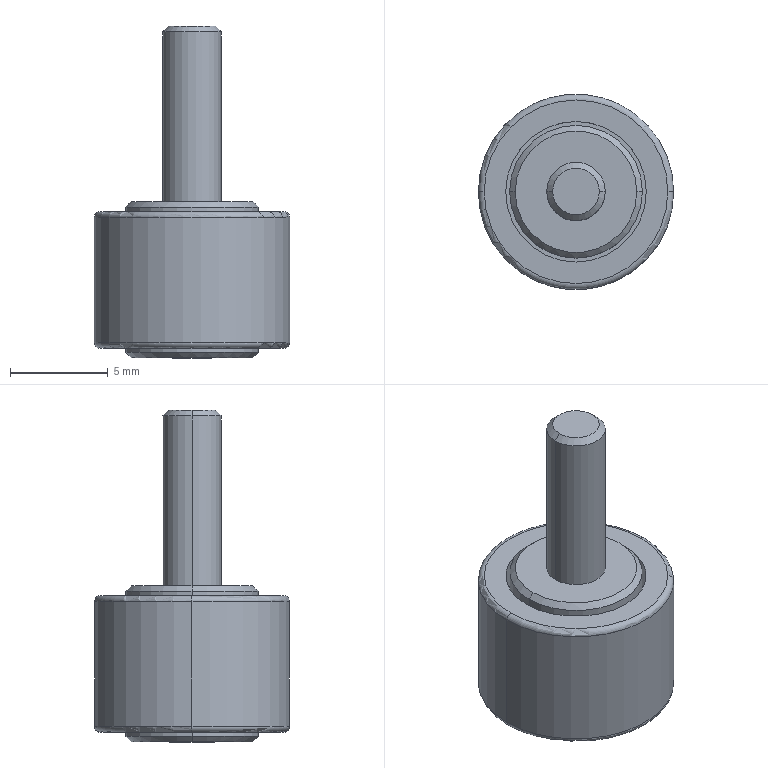Part | NX | features BREP 1 | 1 solid | 36 faces | box 10 x 10 x 17 mm | volume 619.39 mm3 | plane 14 | cylinder 12 | cone 6 | torus 4 | commonest cylinder face diameters 6.8 x4 7.2 x4 3 x2 10 x2
STEP:
#1=CARTESIAN_POINT('',(3.117,0.,-17.));
#2=VERTEX_POINT('',#1);
#3=CARTESIAN_POINT('',(-3.117,0.,-17.));
#4=VERTEX_POINT('',#3);
#5=CARTESIAN_POINT('',(0.,0.,-17.));
#6=DIRECTION('',(0.,0.,1.));
#7=DIRECTION('',(1.,0.,0.));
#8=AXIS2_PLACEMENT_3D('',#5,#6,#7);
#9=CIRCLE('',#8,3.117);
#10=EDGE_CURVE('',#2,#4,#9,.T.);
#11=ORIENTED_EDGE('',*,*,#10,.T.);
#12=CARTESIAN_POINT('',(-3.4,0.,-16.717));
#13=VERTEX_POINT('',#12);
#14=CARTESIAN_POINT('',(-3.117,0.,-17.));
#15=DIRECTION('',(-0.7071,0.,0.7071));
#16=VECTOR('',#15,1000.);
#17=LINE('',#14,#16);
#18=EDGE_CURVE('',#4,#13,#17,.T.);
#19=ORIENTED_EDGE('',*,*,#18,.T.);
#20=CARTESIAN_POINT('',(3.4,0.,-16.717));
#21=VERTEX_POINT('',#20);
#22=CARTESIAN_POINT('',(0.,0.,-16.717));
#23=DIRECTION('',(0.,0.,1.));
#24=DIRECTION('',(1.,0.,0.));
#25=AXIS2_PLACEMENT_3D('',#22,#23,#24);
#26=CIRCLE('',#25,3.4);
#27=EDGE_CURVE('',#21,#13,#26,.T.);
#28=ORIENTED_EDGE('',*,*,#27,.F.);
#29=CARTESIAN_POINT('',(3.117,0.,-17.));
#30=DIRECTION('',(0.7071,0.,0.7071));
#31=VECTOR('',#30,1000.);
#32=LINE('',#29,#31);
#33=EDGE_CURVE('',#2,#21,#32,.T.);
#34=ORIENTED_EDGE('',*,*,#33,.F.);
#35=EDGE_LOOP('',(#11,#19,#28,#34));
#36=FACE_BOUND('',#35,.T.);
#37=CARTESIAN_POINT('',(0.,0.,-17.));
#38=DIRECTION('',(0.,0.,1.));
#39=DIRECTION('',(-1.,0.,0.));
#40=AXIS2_PLACEMENT_3D('',#37,#38,#39);
#41=CONICAL_SURFACE('',#40,3.117,0.7854);
#42=ADVANCED_FACE('',(#36),#41,.T.);
#43=ORIENTED_EDGE('',*,*,#27,.T.);
#44=CARTESIAN_POINT('',(-3.4,0.,-15.));
#45=VERTEX_POINT('',#44);
#46=CARTESIAN_POINT('',(-3.4,0.,-17.));
#47=DIRECTION('',(0.,0.,1.));
#48=VECTOR('',#47,1000.);
#49=LINE('',#46,#48);
#50=EDGE_CURVE('',#13,#45,#49,.T.);
#51=ORIENTED_EDGE('',*,*,#50,.T.);
#52=CARTESIAN_POINT('',(3.4,0.,-15.));
#53=VERTEX_POINT('',#52);
#54=CARTESIAN_POINT('',(0.,0.,-15.));
#55=DIRECTION('',(0.,0.,1.));
#56=DIRECTION('',(1.,0.,0.));
#57=AXIS2_PLACEMENT_3D('',#54,#55,#56);
#58=CIRCLE('',#57,3.4);
#59=EDGE_CURVE('',#53,#45,#58,.T.);
#60=ORIENTED_EDGE('',*,*,#59,.F.);
#61=CARTESIAN_POINT('',(3.4,0.,-17.));
#62=DIRECTION('',(0.,0.,1.));
#63=VECTOR('',#62,1000.);
#64=LINE('',#61,#63);
#65=EDGE_CURVE('',#21,#53,#64,.T.);
#66=ORIENTED_EDGE('',*,*,#65,.F.);
#67=EDGE_LOOP('',(#43,#51,#60,#66));
#68=FACE_BOUND('',#67,.T.);
#69=CARTESIAN_POINT('',(0.,0.,-17.));
#70=DIRECTION('',(0.,0.,1.));
#71=DIRECTION('',(-1.,0.,0.));
#72=AXIS2_PLACEMENT_3D('',#69,#70,#71);
#73=CYLINDRICAL_SURFACE('',#72,3.4);
#74=ADVANCED_FACE('',(#68),#73,.T.);
#75=CARTESIAN_POINT('',(-3.6,0.,-16.5));
#76=VERTEX_POINT('',#75);
#77=CARTESIAN_POINT('',(3.6,0.,-16.5));
#78=VERTEX_POINT('',#77);
#79=CARTESIAN_POINT('',(0.,0.,-16.5));
#80=DIRECTION('',(0.,0.,1.));
#81=DIRECTION('',(1.,0.,0.));
#82=AXIS2_PLACEMENT_3D('',#79,#80,#81);
#83=CIRCLE('',#82,3.6);
#84=EDGE_CURVE('',#76,#78,#83,.T.);
#85=ORIENTED_EDGE('',*,*,#84,.F.);
#86=CARTESIAN_POINT('',(-3.6,0.,-15.));
#87=VERTEX_POINT('',#86);
#88=CARTESIAN_POINT('',(-3.6,0.,-17.));
#89=DIRECTION('',(0.,0.,1.));
#90=VECTOR('',#89,1000.);
#91=LINE('',#88,#90);
#92=EDGE_CURVE('',#76,#87,#91,.T.);
#93=ORIENTED_EDGE('',*,*,#92,.T.);
#94=CARTESIAN_POINT('',(3.6,0.,-15.));
#95=VERTEX_POINT('',#94);
#96=CARTESIAN_POINT('',(0.,0.,-15.));
#97=DIRECTION('',(0.,0.,1.));
#98=DIRECTION('',(1.,0.,0.));
#99=AXIS2_PLACEMENT_3D('',#96,#97,#98);
#100=CIRCLE('',#99,3.6);
#101=EDGE_CURVE('',#87,#95,#100,.T.);
#102=ORIENTED_EDGE('',*,*,#101,.T.);
#103=CARTESIAN_POINT('',(3.6,0.,-17.));
#104=DIRECTION('',(0.,0.,1.));
#105=VECTOR('',#104,1000.);
#106=LINE('',#103,#105);
#107=EDGE_CURVE('',#78,#95,#106,.T.);
#108=ORIENTED_EDGE('',*,*,#107,.F.);
#109=EDGE_LOOP('',(#85,#93,#102,#108));
#110=FACE_BOUND('',#109,.T.);
#111=CARTESIAN_POINT('',(0.,0.,-17.));
#112=DIRECTION('',(0.,0.,1.));
#113=DIRECTION('',(-1.,0.,0.));
#114=AXIS2_PLACEMENT_3D('',#111,#112,#113);
#115=CYLINDRICAL_SURFACE('',#114,3.6);
#116=ADVANCED_FACE('',(#110),#115,.F.);
#117=CARTESIAN_POINT('',(4.7,0.,-16.5));
#118=VERTEX_POINT('',#117);
#119=CARTESIAN_POINT('',(-4.7,0.,-16.5));
#120=VERTEX_POINT('',#119);
#121=CARTESIAN_POINT('',(0.,0.,-16.5));
#122=DIRECTION('',(0.,0.,1.));
#123=DIRECTION('',(1.,0.,0.));
#124=AXIS2_PLACEMENT_3D('',#121,#122,#123);
#125=CIRCLE('',#124,4.7);
#126=EDGE_CURVE('',#118,#120,#125,.T.);
#127=ORIENTED_EDGE('',*,*,#126,.T.);
#128=CARTESIAN_POINT('',(-5.,0.,-16.2));
#129=VERTEX_POINT('',#128);
#130=CARTESIAN_POINT('',(-4.7,0.,-16.2));
#131=DIRECTION('',(0.,1.,0.));
#132=DIRECTION('',(-1.,0.,0.));
#133=AXIS2_PLACEMENT_3D('',#130,#131,#132);
#134=CIRCLE('',#133,0.3);
#135=EDGE_CURVE('',#120,#129,#134,.T.);
#136=ORIENTED_EDGE('',*,*,#135,.T.);
#137=CARTESIAN_POINT('',(5.,0.,-16.2));
#138=VERTEX_POINT('',#137);
#139=CARTESIAN_POINT('',(0.,0.,-16.2));
#140=DIRECTION('',(0.,0.,1.));
#141=DIRECTION('',(1.,0.,0.));
#142=AXIS2_PLACEMENT_3D('',#139,#140,#141);
#143=CIRCLE('',#142,5.);
#144=EDGE_CURVE('',#138,#129,#143,.T.);
#145=ORIENTED_EDGE('',*,*,#144,.F.);
#146=CARTESIAN_POINT('',(4.7,0.,-16.2));
#147=DIRECTION('',(0.,-1.,0.));
#148=DIRECTION('',(0.,0.,-1.));
#149=AXIS2_PLACEMENT_3D('',#146,#147,#148);
#150=CIRCLE('',#149,0.3);
#151=EDGE_CURVE('',#118,#138,#150,.T.);
#152=ORIENTED_EDGE('',*,*,#151,.F.);
#153=EDGE_LOOP('',(#127,#136,#145,#152));
#154=FACE_BOUND('',#153,.T.);
#155=CARTESIAN_POINT('',(0.,0.,-16.2));
#156=DIRECTION('',(0.,0.,1.));
#157=DIRECTION('',(-1.,0.,0.));
#158=AXIS2_PLACEMENT_3D('',#155,#156,#157);
#159=TOROIDAL_SURFACE('',#158,4.7,0.3);
#160=ADVANCED_FACE('',(#154),#159,.T.);
#161=ORIENTED_EDGE('',*,*,#144,.T.);
#162=CARTESIAN_POINT('',(-5.,0.,-9.8));
#163=VERTEX_POINT('',#162);
#164=CARTESIAN_POINT('',(-5.,0.,-17.));
#165=DIRECTION('',(0.,0.,1.));
#166=VECTOR('',#165,1000.);
#167=LINE('',#164,#166);
#168=EDGE_CURVE('',#129,#163,#167,.T.);
#169=ORIENTED_EDGE('',*,*,#168,.T.);
#170=CARTESIAN_POINT('',(5.,0.,-9.8));
#171=VERTEX_POINT('',#170);
#172=CARTESIAN_POINT('',(0.,0.,-9.8));
#173=DIRECTION('',(0.,0.,1.));
#174=DIRECTION('',(1.,0.,0.));
#175=AXIS2_PLACEMENT_3D('',#172,#173,#174);
#176=CIRCLE('',#175,5.);
#177=EDGE_CURVE('',#171,#163,#176,.T.);
#178=ORIENTED_EDGE('',*,*,#177,.F.);
#179=CARTESIAN_POINT('',(5.,0.,-17.));
#180=DIRECTION('',(0.,0.,1.));
#181=VECTOR('',#180,1000.);
#182=LINE('',#179,#181);
#183=EDGE_CURVE('',#138,#171,#182,.T.);
#184=ORIENTED_EDGE('',*,*,#183,.F.);
#185=EDGE_LOOP('',(#161,#169,#178,#184));
#186=FACE_BOUND('',#185,.T.);
#187=CARTESIAN_POINT('',(0.,0.,-17.));
#188=DIRECTION('',(0.,0.,1.));
#189=DIRECTION('',(-1.,0.,0.));
#190=AXIS2_PLACEMENT_3D('',#187,#188,#189);
#191=CYLINDRICAL_SURFACE('',#190,5.);
#192=ADVANCED_FACE('',(#186),#191,.T.);
#193=ORIENTED_EDGE('',*,*,#177,.T.);
#194=CARTESIAN_POINT('',(-4.7,0.,-9.5));
#195=VERTEX_POINT('',#194);
#196=CARTESIAN_POINT('',(-4.7,0.,-9.8));
#197=DIRECTION('',(0.,1.,0.));
#198=DIRECTION('',(-1.,0.,0.));
#199=AXIS2_PLACEMENT_3D('',#196,#197,#198);
#200=CIRCLE('',#199,0.3);
#201=EDGE_CURVE('',#163,#195,#200,.T.);
#202=ORIENTED_EDGE('',*,*,#201,.T.);
#203=CARTESIAN_POINT('',(4.7,0.,-9.5));
#204=VERTEX_POINT('',#203);
#205=CARTESIAN_POINT('',(0.,0.,-9.5));
#206=DIRECTION('',(0.,0.,1.));
#207=DIRECTION('',(1.,0.,0.));
#208=AXIS2_PLACEMENT_3D('',#205,#206,#207);
#209=CIRCLE('',#208,4.7);
#210=EDGE_CURVE('',#204,#195,#209,.T.);
#211=ORIENTED_EDGE('',*,*,#210,.F.);
#212=CARTESIAN_POINT('',(4.7,0.,-9.8));
#213=DIRECTION('',(0.,-1.,0.));
#214=DIRECTION('',(0.,0.,-1.));
#215=AXIS2_PLACEMENT_3D('',#212,#213,#214);
#216=CIRCLE('',#215,0.3);
#217=EDGE_CURVE('',#171,#204,#216,.T.);
#218=ORIENTED_EDGE('',*,*,#217,.F.);
#219=EDGE_LOOP('',(#193,#202,#211,#218));
#220=FACE_BOUND('',#219,.T.);
#221=CARTESIAN_POINT('',(0.,0.,-9.8));
#222=DIRECTION('',(0.,0.,1.));
#223=DIRECTION('',(-1.,0.,0.));
#224=AXIS2_PLACEMENT_3D('',#221,#222,#223);
#225=TOROIDAL_SURFACE('',#224,4.7,0.3);
#226=ADVANCED_FACE('',(#220),#225,.T.);
#227=CARTESIAN_POINT('',(-3.6,0.,-11.));
#228=VERTEX_POINT('',#227);
#229=CARTESIAN_POINT('',(3.6,0.,-11.));
#230=VERTEX_POINT('',#229);
#231=CARTESIAN_POINT('',(0.,0.,-11.));
#232=DIRECTION('',(0.,0.,1.));
#233=DIRECTION('',(1.,0.,0.));
#234=AXIS2_PLACEMENT_3D('',#231,#232,#233);
#235=CIRCLE('',#234,3.6);
#236=EDGE_CURVE('',#228,#230,#235,.T.);
#237=ORIENTED_EDGE('',*,*,#236,.F.);
#238=CARTESIAN_POINT('',(-3.6,0.,-9.5));
#239=VERTEX_POINT('',#238);
#240=CARTESIAN_POINT('',(-3.6,0.,-17.));
#241=DIRECTION('',(0.,0.,1.));
#242=VECTOR('',#241,1000.);
#243=LINE('',#240,#242);
#244=EDGE_CURVE('',#228,#239,#243,.T.);
#245=ORIENTED_EDGE('',*,*,#244,.T.);
#246=CARTESIAN_POINT('',(3.6,0.,-9.5));
#247=VERTEX_POINT('',#246);
#248=CARTESIAN_POINT('',(0.,0.,-9.5));
#249=DIRECTION('',(0.,0.,1.));
#250=DIRECTION('',(1.,0.,0.));
#251=AXIS2_PLACEMENT_3D('',#248,#249,#250);
#252=CIRCLE('',#251,3.6);
#253=EDGE_CURVE('',#239,#247,#252,.T.);
#254=ORIENTED_EDGE('',*,*,#253,.T.);
#255=CARTESIAN_POINT('',(3.6,0.,-17.));
#256=DIRECTION('',(0.,0.,1.));
#257=VECTOR('',#256,1000.);
#258=LINE('',#255,#257);
#259=EDGE_CURVE('',#230,#247,#258,.T.);
#260=ORIENTED_EDGE('',*,*,#259,.F.);
#261=EDGE_LOOP('',(#237,#245,#254,#260));
#262=FACE_BOUND('',#261,.T.);
#263=CARTESIAN_POINT('',(0.,0.,-17.));
#264=DIRECTION('',(0.,0.,1.));
#265=DIRECTION('',(-1.,0.,0.));
#266=AXIS2_PLACEMENT_3D('',#263,#264,#265);
#267=CYLINDRICAL_SURFACE('',#266,3.6);
#268=ADVANCED_FACE('',(#262),#267,.F.);
#269=CARTESIAN_POINT('',(3.4,0.,-11.));
#270=VERTEX_POINT('',#269);
#271=CARTESIAN_POINT('',(-3.4,0.,-11.));
#272=VERTEX_POINT('',#271);
#273=CARTESIAN_POINT('',(0.,0.,-11.));
#274=DIRECTION('',(0.,0.,1.));
#275=DIRECTION('',(1.,0.,0.));
#276=AXIS2_PLACEMENT_3D('',#273,#274,#275);
#277=CIRCLE('',#276,3.4);
#278=EDGE_CURVE('',#270,#272,#277,.T.);
#279=ORIENTED_EDGE('',*,*,#278,.T.);
#280=CARTESIAN_POINT('',(-3.4,0.,-9.283));
#281=VERTEX_POINT('',#280);
#282=CARTESIAN_POINT('',(-3.4,0.,-17.));
#283=DIRECTION('',(0.,0.,1.));
#284=VECTOR('',#283,1000.);
#285=LINE('',#282,#284);
#286=EDGE_CURVE('',#272,#281,#285,.T.);
#287=ORIENTED_EDGE('',*,*,#286,.T.);
#288=CARTESIAN_POINT('',(3.4,0.,-9.283));
#289=VERTEX_POINT('',#288);
#290=CARTESIAN_POINT('',(0.,0.,-9.283));
#291=DIRECTION('',(0.,0.,1.));
#292=DIRECTION('',(1.,0.,0.));
#293=AXIS2_PLACEMENT_3D('',#290,#291,#292);
#294=CIRCLE('',#293,3.4);
#295=EDGE_CURVE('',#289,#281,#294,.T.);
#296=ORIENTED_EDGE('',*,*,#295,.F.);
#297=CARTESIAN_POINT('',(3.4,0.,-17.));
#298=DIRECTION('',(0.,0.,1.));
#299=VECTOR('',#298,1000.);
#300=LINE('',#297,#299);
#301=EDGE_CURVE('',#270,#289,#300,.T.);
#302=ORIENTED_EDGE('',*,*,#301,.F.);
#303=EDGE_LOOP('',(#279,#287,#296,#302));
#304=FACE_BOUND('',#303,.T.);
#305=CARTESIAN_POINT('',(0.,0.,-17.));
#306=DIRECTION('',(0.,0.,1.));
#307=DIRECTION('',(-1.,0.,0.));
#308=AXIS2_PLACEMENT_3D('',#305,#306,#307);
#309=CYLINDRICAL_SURFACE('',#308,3.4);
#310=ADVANCED_FACE('',(#304),#309,.T.);
#311=CARTESIAN_POINT('',(3.117,0.,-9.));
#312=VERTEX_POINT('',#311);
#313=CARTESIAN_POINT('',(-3.117,0.,-9.));
#314=VERTEX_POINT('',#313);
#315=CARTESIAN_POINT('',(0.,0.,-9.));
#316=DIRECTION('',(0.,0.,1.));
#317=DIRECTION('',(1.,0.,0.));
#318=AXIS2_PLACEMENT_3D('',#315,#316,#317);
#319=CIRCLE('',#318,3.117);
#320=EDGE_CURVE('',#312,#314,#319,.T.);
#321=ORIENTED_EDGE('',*,*,#320,.F.);
#322=CARTESIAN_POINT('',(3.4,0.,-9.283));
#323=DIRECTION('',(0.7071,0.,-0.7071));
#324=VECTOR('',#323,1000.);
#325=LINE('',#322,#324);
#326=EDGE_CURVE('',#289,#312,#325,.F.);
#327=ORIENTED_EDGE('',*,*,#326,.F.);
#328=ORIENTED_EDGE('',*,*,#295,.T.);
#329=CARTESIAN_POINT('',(-3.4,0.,-9.283));
#330=DIRECTION('',(-0.7071,0.,-0.7071));
#331=VECTOR('',#330,1000.);
#332=LINE('',#329,#331);
#333=EDGE_CURVE('',#281,#314,#332,.F.);
#334=ORIENTED_EDGE('',*,*,#333,.T.);
#335=EDGE_LOOP('',(#321,#327,#328,#334));
#336=FACE_BOUND('',#335,.T.);
#337=CARTESIAN_POINT('',(0.,0.,-9.283));
#338=DIRECTION('',(0.,0.,-1.));
#339=DIRECTION('',(1.,0.,0.));
#340=AXIS2_PLACEMENT_3D('',#337,#338,#339);
#341=CONICAL_SURFACE('',#340,3.4,0.7854);
#342=ADVANCED_FACE('',(#336),#341,.T.);
#343=CARTESIAN_POINT('',(1.5,0.,-9.));
#344=VERTEX_POINT('',#343);
#345=CARTESIAN_POINT('',(-1.5,0.,-9.));
#346=VERTEX_POINT('',#345);
#347=CARTESIAN_POINT('',(0.,0.,-9.));
#348=DIRECTION('',(0.,0.,1.));
#349=DIRECTION('',(1.,0.,0.));
#350=AXIS2_PLACEMENT_3D('',#347,#348,#349);
#351=CIRCLE('',#350,1.5);
#352=EDGE_CURVE('',#344,#346,#351,.T.);
#353=ORIENTED_EDGE('',*,*,#352,.T.);
#354=CARTESIAN_POINT('',(-1.5,0.,-0.3065));
#355=VERTEX_POINT('',#354);
#356=CARTESIAN_POINT('',(-1.5,0.,-17.));
#357=DIRECTION('',(0.,0.,1.));
#358=VECTOR('',#357,1000.);
#359=LINE('',#356,#358);
#360=EDGE_CURVE('',#346,#355,#359,.T.);
#361=ORIENTED_EDGE('',*,*,#360,.T.);
#362=CARTESIAN_POINT('',(1.5,0.,-0.3065));
#363=VERTEX_POINT('',#362);
#364=CARTESIAN_POINT('',(0.,0.,-0.3065));
#365=DIRECTION('',(0.,0.,1.));
#366=DIRECTION('',(1.,0.,0.));
#367=AXIS2_PLACEMENT_3D('',#364,#365,#366);
#368=CIRCLE('',#367,1.5);
#369=EDGE_CURVE('',#363,#355,#368,.T.);
#370=ORIENTED_EDGE('',*,*,#369,.F.);
#371=CARTESIAN_POINT('',(1.5,0.,-17.));
#372=DIRECTION('',(0.,0.,1.));
#373=VECTOR('',#372,1000.);
#374=LINE('',#371,#373);
#375=EDGE_CURVE('',#344,#363,#374,.T.);
#376=ORIENTED_EDGE('',*,*,#375,.F.);
#377=EDGE_LOOP('',(#353,#361,#370,#376));
#378=FACE_BOUND('',#377,.T.);
#379=CARTESIAN_POINT('',(0.,0.,-17.));
#380=DIRECTION('',(0.,0.,1.));
#381=DIRECTION('',(-1.,0.,0.));
#382=AXIS2_PLACEMENT_3D('',#379,#380,#381);
#383=CYLINDRICAL_SURFACE('',#382,1.5);
#384=ADVANCED_FACE('',(#378),#383,.T.);
#385=CARTESIAN_POINT('',(1.194,0.,0.));
#386=VERTEX_POINT('',#385);
#387=CARTESIAN_POINT('',(-1.194,0.,0.));
#388=VERTEX_POINT('',#387);
#389=CARTESIAN_POINT('',(0.,0.,0.));
#390=DIRECTION('',(0.,0.,1.));
#391=DIRECTION('',(1.,0.,0.));
#392=AXIS2_PLACEMENT_3D('',#389,#390,#391);
#393=CIRCLE('',#392,1.194);
#394=EDGE_CURVE('',#386,#388,#393,.T.);
#395=ORIENTED_EDGE('',*,*,#394,.F.);
#396=CARTESIAN_POINT('',(1.5,0.,-0.3065));
#397=DIRECTION('',(0.7071,0.,-0.7071));
#398=VECTOR('',#397,1000.);
#399=LINE('',#396,#398);
#400=EDGE_CURVE('',#363,#386,#399,.F.);
#401=ORIENTED_EDGE('',*,*,#400,.F.);
#402=ORIENTED_EDGE('',*,*,#369,.T.);
#403=CARTESIAN_POINT('',(-1.5,0.,-0.3065));
#404=DIRECTION('',(-0.7071,0.,-0.7071));
#405=VECTOR('',#404,1000.);
#406=LINE('',#403,#405);
#407=EDGE_CURVE('',#355,#388,#406,.F.);
#408=ORIENTED_EDGE('',*,*,#407,.T.);
#409=EDGE_LOOP('',(#395,#401,#402,#408));
#410=FACE_BOUND('',#409,.T.);
#411=CARTESIAN_POINT('',(0.,0.,-0.3065));
#412=DIRECTION('',(0.,0.,-1.));
#413=DIRECTION('',(1.,0.,0.));
#414=AXIS2_PLACEMENT_3D('',#411,#412,#413);
#415=CONICAL_SURFACE('',#414,1.5,0.7854);
#416=ADVANCED_FACE('',(#410),#415,.T.);
#417=ORIENTED_EDGE('',*,*,#10,.F.);
#418=CARTESIAN_POINT('',(0.,0.,-17.));
#419=DIRECTION('',(0.,0.,1.));
#420=DIRECTION('',(1.,0.,0.));
#421=AXIS2_PLACEMENT_3D('',#418,#419,#420);
#422=CIRCLE('',#421,3.117);
#423=EDGE_CURVE('',#4,#2,#422,.T.);
#424=ORIENTED_EDGE('',*,*,#423,.F.);
#425=EDGE_LOOP('',(#417,#424));
#426=FACE_BOUND('',#425,.T.);
#427=CARTESIAN_POINT('',(-1.,0.5774,-17.));
#428=VERTEX_POINT('',#427);
#429=CARTESIAN_POINT('',(-1.,-0.5774,-17.));
#430=VERTEX_POINT('',#429);
#431=CARTESIAN_POINT('',(-1.,0.5774,-17.));
#432=DIRECTION('',(0.,-1.,0.));
#433=VECTOR('',#432,1000.);
#434=LINE('',#431,#433);
#435=EDGE_CURVE('',#428,#430,#434,.T.);
#436=ORIENTED_EDGE('',*,*,#435,.T.);
#437=CARTESIAN_POINT('',(0.,-1.155,-17.));
#438=VERTEX_POINT('',#437);
#439=CARTESIAN_POINT('',(-1.,-0.5774,-17.));
#440=DIRECTION('',(0.866,-0.5,0.));
#441=VECTOR('',#440,1000.);
#442=LINE('',#439,#441);
#443=EDGE_CURVE('',#430,#438,#442,.T.);
#444=ORIENTED_EDGE('',*,*,#443,.T.);
#445=CARTESIAN_POINT('',(1.,-0.5774,-17.));
#446=VERTEX_POINT('',#445);
#447=CARTESIAN_POINT('',(0.,-1.155,-17.));
#448=DIRECTION('',(0.866,0.5,0.));
#449=VECTOR('',#448,1000.);
#450=LINE('',#447,#449);
#451=EDGE_CURVE('',#438,#446,#450,.T.);
#452=ORIENTED_EDGE('',*,*,#451,.T.);
#453=CARTESIAN_POINT('',(1.,0.5774,-17.));
#454=VERTEX_POINT('',#453);
#455=CARTESIAN_POINT('',(1.,-0.5774,-17.));
#456=DIRECTION('',(0.,1.,0.));
#457=VECTOR('',#456,1000.);
#458=LINE('',#455,#457);
#459=EDGE_CURVE('',#446,#454,#458,.T.);
#460=ORIENTED_EDGE('',*,*,#459,.T.);
#461=CARTESIAN_POINT('',(0.,1.155,-17.));
#462=VERTEX_POINT('',#461);
#463=CARTESIAN_POINT('',(1.,0.5774,-17.));
#464=DIRECTION('',(-0.866,0.5,0.));
#465=VECTOR('',#464,1000.);
#466=LINE('',#463,#465);
#467=EDGE_CURVE('',#454,#462,#466,.T.);
#468=ORIENTED_EDGE('',*,*,#467,.T.);
#469=CARTESIAN_POINT('',(0.,1.155,-17.));
#470=DIRECTION('',(-0.866,-0.5,0.));
#471=VECTOR('',#470,1000.);
#472=LINE('',#469,#471);
#473=EDGE_CURVE('',#462,#428,#472,.T.);
#474=ORIENTED_EDGE('',*,*,#473,.T.);
#475=EDGE_LOOP('',(#436,#444,#452,#460,#468,#474));
#476=FACE_BOUND('',#475,.T.);
#477=CARTESIAN_POINT('',(0.,3.117,-17.));
#478=DIRECTION('',(0.,0.,1.));
#479=DIRECTION('',(-1.,0.,0.));
#480=AXIS2_PLACEMENT_3D('',#477,#478,#479);
#481=PLANE('',#480);
#482=ADVANCED_FACE('',(#426,#476),#481,.F.);
#483=CARTESIAN_POINT('',(0.,0.,0.));
#484=DIRECTION('',(0.,0.,1.));
#485=DIRECTION('',(1.,0.,0.));
#486=AXIS2_PLACEMENT_3D('',#483,#484,#485);
#487=CIRCLE('',#486,1.194);
#488=EDGE_CURVE('',#388,#386,#487,.T.);
#489=ORIENTED_EDGE('',*,*,#488,.T.);
#490=ORIENTED_EDGE('',*,*,#394,.T.);
#491=EDGE_LOOP('',(#489,#490));
#492=FACE_BOUND('',#491,.T.);
#493=CARTESIAN_POINT('',(0.,0.,0.));
#494=DIRECTION('',(0.,0.,-1.));
#495=DIRECTION('',(1.,0.,0.));
#496=AXIS2_PLACEMENT_3D('',#493,#494,#495);
#497=PLANE('',#496);
#498=ADVANCED_FACE('',(#492),#497,.F.);
#499=ORIENTED_EDGE('',*,*,#400,.T.);
#500=ORIENTED_EDGE('',*,*,#488,.F.);
#501=ORIENTED_EDGE('',*,*,#407,.F.);
#502=CARTESIAN_POINT('',(0.,0.,-0.3065));
#503=DIRECTION('',(0.,0.,1.));
#504=DIRECTION('',(1.,0.,0.));
#505=AXIS2_PLACEMENT_3D('',#502,#503,#504);
#506=CIRCLE('',#505,1.5);
#507=EDGE_CURVE('',#355,#363,#506,.T.);
#508=ORIENTED_EDGE('',*,*,#507,.T.);
#509=EDGE_LOOP('',(#499,#500,#501,#508));
#510=FACE_BOUND('',#509,.T.);
#511=CARTESIAN_POINT('',(0.,0.,-0.3065));
#512=DIRECTION('',(0.,0.,-1.));
#513=DIRECTION('',(1.,0.,0.));
#514=AXIS2_PLACEMENT_3D('',#511,#512,#513);
#515=CONICAL_SURFACE('',#514,1.5,0.7854);
#516=ADVANCED_FACE('',(#510),#515,.T.);
#517=ORIENTED_EDGE('',*,*,#360,.F.);
#518=CARTESIAN_POINT('',(0.,0.,-9.));
#519=DIRECTION('',(0.,0.,1.));
#520=DIRECTION('',(1.,0.,0.));
#521=AXIS2_PLACEMENT_3D('',#518,#519,#520);
#522=CIRCLE('',#521,1.5);
#523=EDGE_CURVE('',#346,#344,#522,.T.);
#524=ORIENTED_EDGE('',*,*,#523,.T.);
#525=ORIENTED_EDGE('',*,*,#375,.T.);
#526=ORIENTED_EDGE('',*,*,#507,.F.);
#527=EDGE_LOOP('',(#517,#524,#525,#526));
#528=FACE_BOUND('',#527,.T.);
#529=CARTESIAN_POINT('',(0.,0.,-17.));
#530=DIRECTION('',(0.,0.,1.));
#531=DIRECTION('',(-1.,0.,0.));
#532=AXIS2_PLACEMENT_3D('',#529,#530,#531);
#533=CYLINDRICAL_SURFACE('',#532,1.5);
#534=ADVANCED_FACE('',(#528),#533,.T.);
#535=ORIENTED_EDGE('',*,*,#352,.F.);
#536=ORIENTED_EDGE('',*,*,#523,.F.);
#537=EDGE_LOOP('',(#535,#536));
#538=FACE_BOUND('',#537,.T.);
#539=CARTESIAN_POINT('',(0.,0.,-9.));
#540=DIRECTION('',(0.,0.,1.));
#541=DIRECTION('',(1.,0.,0.));
#542=AXIS2_PLACEMENT_3D('',#539,#540,#541);
#543=CIRCLE('',#542,3.117);
#544=EDGE_CURVE('',#314,#312,#543,.T.);
#545=ORIENTED_EDGE('',*,*,#544,.T.);
#546=ORIENTED_EDGE('',*,*,#320,.T.);
#547=EDGE_LOOP('',(#545,#546));
#548=FACE_BOUND('',#547,.T.);
#549=CARTESIAN_POINT('',(0.,1.5,-9.));
#550=DIRECTION('',(0.,0.,-1.));
#551=DIRECTION('',(1.,0.,0.));
#552=AXIS2_PLACEMENT_3D('',#549,#550,#551);
#553=PLANE('',#552);
#554=ADVANCED_FACE('',(#538,#548),#553,.F.);
#555=ORIENTED_EDGE('',*,*,#326,.T.);
#556=ORIENTED_EDGE('',*,*,#544,.F.);
#557=ORIENTED_EDGE('',*,*,#333,.F.);
#558=CARTESIAN_POINT('',(0.,0.,-9.283));
#559=DIRECTION('',(0.,0.,1.));
#560=DIRECTION('',(1.,0.,0.));
#561=AXIS2_PLACEMENT_3D('',#558,#559,#560);
#562=CIRCLE('',#561,3.4);
#563=EDGE_CURVE('',#281,#289,#562,.T.);
#564=ORIENTED_EDGE('',*,*,#563,.T.);
#565=EDGE_LOOP('',(#555,#556,#557,#564));
#566=FACE_BOUND('',#565,.T.);
#567=CARTESIAN_POINT('',(0.,0.,-9.283));
#568=DIRECTION('',(0.,0.,-1.));
#569=DIRECTION('',(1.,0.,0.));
#570=AXIS2_PLACEMENT_3D('',#567,#568,#569);
#571=CONICAL_SURFACE('',#570,3.4,0.7854);
#572=ADVANCED_FACE('',(#566),#571,.T.);
#573=ORIENTED_EDGE('',*,*,#286,.F.);
#574=CARTESIAN_POINT('',(0.,0.,-11.));
#575=DIRECTION('',(0.,0.,1.));
#576=DIRECTION('',(1.,0.,0.));
#577=AXIS2_PLACEMENT_3D('',#574,#575,#576);
#578=CIRCLE('',#577,3.4);
#579=EDGE_CURVE('',#272,#270,#578,.T.);
#580=ORIENTED_EDGE('',*,*,#579,.T.);
#581=ORIENTED_EDGE('',*,*,#301,.T.);
#582=ORIENTED_EDGE('',*,*,#563,.F.);
#583=EDGE_LOOP('',(#573,#580,#581,#582));
#584=FACE_BOUND('',#583,.T.);
#585=CARTESIAN_POINT('',(0.,0.,-17.));
#586=DIRECTION('',(0.,0.,1.));
#587=DIRECTION('',(-1.,0.,0.));
#588=AXIS2_PLACEMENT_3D('',#585,#586,#587);
#589=CYLINDRICAL_SURFACE('',#588,3.4);
#590=ADVANCED_FACE('',(#584),#589,.T.);
#591=ORIENTED_EDGE('',*,*,#278,.F.);
#592=ORIENTED_EDGE('',*,*,#579,.F.);
#593=EDGE_LOOP('',(#591,#592));
#594=FACE_BOUND('',#593,.T.);
#595=CARTESIAN_POINT('',(0.,0.,-11.));
#596=DIRECTION('',(0.,0.,1.));
#597=DIRECTION('',(1.,0.,0.));
#598=AXIS2_PLACEMENT_3D('',#595,#596,#597);
#599=CIRCLE('',#598,3.6);
#600=EDGE_CURVE('',#230,#228,#599,.T.);
#601=ORIENTED_EDGE('',*,*,#600,.T.);
#602=ORIENTED_EDGE('',*,*,#236,.T.);
#603=EDGE_LOOP('',(#601,#602));
#604=FACE_BOUND('',#603,.T.);
#605=CARTESIAN_POINT('',(0.,3.4,-11.));
#606=DIRECTION('',(0.,0.,-1.));
#607=DIRECTION('',(1.,0.,0.));
#608=AXIS2_PLACEMENT_3D('',#605,#606,#607);
#609=PLANE('',#608);
#610=ADVANCED_FACE('',(#594,#604),#609,.F.);
#611=ORIENTED_EDGE('',*,*,#244,.F.);
#612=ORIENTED_EDGE('',*,*,#600,.F.);
#613=ORIENTED_EDGE('',*,*,#259,.T.);
#614=CARTESIAN_POINT('',(0.,0.,-9.5));
#615=DIRECTION('',(0.,0.,1.));
#616=DIRECTION('',(1.,0.,0.));
#617=AXIS2_PLACEMENT_3D('',#614,#615,#616);
#618=CIRCLE('',#617,3.6);
#619=EDGE_CURVE('',#247,#239,#618,.T.);
#620=ORIENTED_EDGE('',*,*,#619,.T.);
#621=EDGE_LOOP('',(#611,#612,#613,#620));
#622=FACE_BOUND('',#621,.T.);
#623=CARTESIAN_POINT('',(0.,0.,-17.));
#624=DIRECTION('',(0.,0.,1.));
#625=DIRECTION('',(-1.,0.,0.));
#626=AXIS2_PLACEMENT_3D('',#623,#624,#625);
#627=CYLINDRICAL_SURFACE('',#626,3.6);
#628=ADVANCED_FACE('',(#622),#627,.F.);
#629=ORIENTED_EDGE('',*,*,#619,.F.);
#630=ORIENTED_EDGE('',*,*,#253,.F.);
#631=EDGE_LOOP('',(#629,#630));
#632=FACE_BOUND('',#631,.T.);
#633=ORIENTED_EDGE('',*,*,#210,.T.);
#634=CARTESIAN_POINT('',(0.,0.,-9.5));
#635=DIRECTION('',(0.,0.,1.));
#636=DIRECTION('',(1.,0.,0.));
#637=AXIS2_PLACEMENT_3D('',#634,#635,#636);
#638=CIRCLE('',#637,4.7);
#639=EDGE_CURVE('',#195,#204,#638,.T.);
#640=ORIENTED_EDGE('',*,*,#639,.T.);
#641=EDGE_LOOP('',(#633,#640));
#642=FACE_BOUND('',#641,.T.);
#643=CARTESIAN_POINT('',(0.,3.6,-9.5));
#644=DIRECTION('',(0.,0.,-1.));
#645=DIRECTION('',(1.,0.,0.));
#646=AXIS2_PLACEMENT_3D('',#643,#644,#645);
#647=PLANE('',#646);
#648=ADVANCED_FACE('',(#632,#642),#647,.F.);
#649=ORIENTED_EDGE('',*,*,#201,.F.);
#650=CARTESIAN_POINT('',(0.,0.,-9.8));
#651=DIRECTION('',(0.,0.,1.));
#652=DIRECTION('',(1.,0.,0.));
#653=AXIS2_PLACEMENT_3D('',#650,#651,#652);
#654=CIRCLE('',#653,5.);
#655=EDGE_CURVE('',#163,#171,#654,.T.);
#656=ORIENTED_EDGE('',*,*,#655,.T.);
#657=ORIENTED_EDGE('',*,*,#217,.T.);
#658=ORIENTED_EDGE('',*,*,#639,.F.);
#659=EDGE_LOOP('',(#649,#656,#657,#658));
#660=FACE_BOUND('',#659,.T.);
#661=CARTESIAN_POINT('',(0.,0.,-9.8));
#662=DIRECTION('',(0.,0.,1.));
#663=DIRECTION('',(-1.,0.,0.));
#664=AXIS2_PLACEMENT_3D('',#661,#662,#663);
#665=TOROIDAL_SURFACE('',#664,4.7,0.3);
#666=ADVANCED_FACE('',(#660),#665,.T.);
#667=ORIENTED_EDGE('',*,*,#168,.F.);
#668=CARTESIAN_POINT('',(0.,0.,-16.2));
#669=DIRECTION('',(0.,0.,1.));
#670=DIRECTION('',(1.,0.,0.));
#671=AXIS2_PLACEMENT_3D('',#668,#669,#670);
#672=CIRCLE('',#671,5.);
#673=EDGE_CURVE('',#129,#138,#672,.T.);
#674=ORIENTED_EDGE('',*,*,#673,.T.);
#675=ORIENTED_EDGE('',*,*,#183,.T.);
#676=ORIENTED_EDGE('',*,*,#655,.F.);
#677=EDGE_LOOP('',(#667,#674,#675,#676));
#678=FACE_BOUND('',#677,.T.);
#679=CARTESIAN_POINT('',(0.,0.,-17.));
#680=DIRECTION('',(0.,0.,1.));
#681=DIRECTION('',(-1.,0.,0.));
#682=AXIS2_PLACEMENT_3D('',#679,#680,#681);
#683=CYLINDRICAL_SURFACE('',#682,5.);
#684=ADVANCED_FACE('',(#678),#683,.T.);
#685=ORIENTED_EDGE('',*,*,#135,.F.);
#686=CARTESIAN_POINT('',(0.,0.,-16.5));
#687=DIRECTION('',(0.,0.,1.));
#688=DIRECTION('',(1.,0.,0.));
#689=AXIS2_PLACEMENT_3D('',#686,#687,#688);
#690=CIRCLE('',#689,4.7);
#691=EDGE_CURVE('',#120,#118,#690,.T.);
#692=ORIENTED_EDGE('',*,*,#691,.T.);
#693=ORIENTED_EDGE('',*,*,#151,.T.);
#694=ORIENTED_EDGE('',*,*,#673,.F.);
#695=EDGE_LOOP('',(#685,#692,#693,#694));
#696=FACE_BOUND('',#695,.T.);
#697=CARTESIAN_POINT('',(0.,0.,-16.2));
#698=DIRECTION('',(0.,0.,1.));
#699=DIRECTION('',(-1.,0.,0.));
#700=AXIS2_PLACEMENT_3D('',#697,#698,#699);
#701=TOROIDAL_SURFACE('',#700,4.7,0.3);
#702=ADVANCED_FACE('',(#696),#701,.T.);
#703=ORIENTED_EDGE('',*,*,#126,.F.);
#704=ORIENTED_EDGE('',*,*,#691,.F.);
#705=EDGE_LOOP('',(#703,#704));
#706=FACE_BOUND('',#705,.T.);
#707=CARTESIAN_POINT('',(0.,0.,-16.5));
#708=DIRECTION('',(0.,0.,1.));
#709=DIRECTION('',(1.,0.,0.));
#710=AXIS2_PLACEMENT_3D('',#707,#708,#709);
#711=CIRCLE('',#710,3.6);
#712=EDGE_CURVE('',#78,#76,#711,.T.);
#713=ORIENTED_EDGE('',*,*,#712,.T.);
#714=ORIENTED_EDGE('',*,*,#84,.T.);
#715=EDGE_LOOP('',(#713,#714));
#716=FACE_BOUND('',#715,.T.);
#717=CARTESIAN_POINT('',(0.,4.7,-16.5));
#718=DIRECTION('',(0.,0.,1.));
#719=DIRECTION('',(-1.,0.,0.));
#720=AXIS2_PLACEMENT_3D('',#717,#718,#719);
#721=PLANE('',#720);
#722=ADVANCED_FACE('',(#706,#716),#721,.F.);
#723=ORIENTED_EDGE('',*,*,#92,.F.);
#724=ORIENTED_EDGE('',*,*,#712,.F.);
#725=ORIENTED_EDGE('',*,*,#107,.T.);
#726=CARTESIAN_POINT('',(0.,0.,-15.));
#727=DIRECTION('',(0.,0.,1.));
#728=DIRECTION('',(1.,0.,0.));
#729=AXIS2_PLACEMENT_3D('',#726,#727,#728);
#730=CIRCLE('',#729,3.6);
#731=EDGE_CURVE('',#95,#87,#730,.T.);
#732=ORIENTED_EDGE('',*,*,#731,.T.);
#733=EDGE_LOOP('',(#723,#724,#725,#732));
#734=FACE_BOUND('',#733,.T.);
#735=CARTESIAN_POINT('',(0.,0.,-17.));
#736=DIRECTION('',(0.,0.,1.));
#737=DIRECTION('',(-1.,0.,0.));
#738=AXIS2_PLACEMENT_3D('',#735,#736,#737);
#739=CYLINDRICAL_SURFACE('',#738,3.6);
#740=ADVANCED_FACE('',(#734),#739,.F.);
#741=ORIENTED_EDGE('',*,*,#731,.F.);
#742=ORIENTED_EDGE('',*,*,#101,.F.);
#743=EDGE_LOOP('',(#741,#742));
#744=FACE_BOUND('',#743,.T.);
#745=ORIENTED_EDGE('',*,*,#59,.T.);
#746=CARTESIAN_POINT('',(0.,0.,-15.));
#747=DIRECTION('',(0.,0.,1.));
#748=DIRECTION('',(1.,0.,0.));
#749=AXIS2_PLACEMENT_3D('',#746,#747,#748);
#750=CIRCLE('',#749,3.4);
#751=EDGE_CURVE('',#45,#53,#750,.T.);
#752=ORIENTED_EDGE('',*,*,#751,.T.);
#753=EDGE_LOOP('',(#745,#752));
#754=FACE_BOUND('',#753,.T.);
#755=CARTESIAN_POINT('',(0.,3.6,-15.));
#756=DIRECTION('',(0.,0.,1.));
#757=DIRECTION('',(-1.,0.,0.));
#758=AXIS2_PLACEMENT_3D('',#755,#756,#757);
#759=PLANE('',#758);
#760=ADVANCED_FACE('',(#744,#754),#759,.F.);
#761=ORIENTED_EDGE('',*,*,#50,.F.);
#762=CARTESIAN_POINT('',(0.,0.,-16.717));
#763=DIRECTION('',(0.,0.,1.));
#764=DIRECTION('',(1.,0.,0.));
#765=AXIS2_PLACEMENT_3D('',#762,#763,#764);
#766=CIRCLE('',#765,3.4);
#767=EDGE_CURVE('',#13,#21,#766,.T.);
#768=ORIENTED_EDGE('',*,*,#767,.T.);
#769=ORIENTED_EDGE('',*,*,#65,.T.);
#770=ORIENTED_EDGE('',*,*,#751,.F.);
#771=EDGE_LOOP('',(#761,#768,#769,#770));
#772=FACE_BOUND('',#771,.T.);
#773=CARTESIAN_POINT('',(0.,0.,-17.));
#774=DIRECTION('',(0.,0.,1.));
#775=DIRECTION('',(-1.,0.,0.));
#776=AXIS2_PLACEMENT_3D('',#773,#774,#775);
#777=CYLINDRICAL_SURFACE('',#776,3.4);
#778=ADVANCED_FACE('',(#772),#777,.T.);
#779=ORIENTED_EDGE('',*,*,#18,.F.);
#780=ORIENTED_EDGE('',*,*,#423,.T.);
#781=ORIENTED_EDGE('',*,*,#33,.T.);
#782=ORIENTED_EDGE('',*,*,#767,.F.);
#783=EDGE_LOOP('',(#779,#780,#781,#782));
#784=FACE_BOUND('',#783,.T.);
#785=CARTESIAN_POINT('',(0.,0.,-17.));
#786=DIRECTION('',(0.,0.,1.));
#787=DIRECTION('',(-1.,0.,0.));
#788=AXIS2_PLACEMENT_3D('',#785,#786,#787);
#789=CONICAL_SURFACE('',#788,3.117,0.7854);
#790=ADVANCED_FACE('',(#784),#789,.T.);
#791=ORIENTED_EDGE('',*,*,#435,.F.);
#792=CARTESIAN_POINT('',(-1.,0.5774,-13.));
#793=VERTEX_POINT('',#792);
#794=CARTESIAN_POINT('',(-1.,0.5774,-13.));
#795=DIRECTION('',(0.,0.,-1.));
#796=VECTOR('',#795,1000.);
#797=LINE('',#794,#796);
#798=EDGE_CURVE('',#793,#428,#797,.T.);
#799=ORIENTED_EDGE('',*,*,#798,.F.);
#800=CARTESIAN_POINT('',(-1.,-0.5774,-13.));
#801=VERTEX_POINT('',#800);
#802=CARTESIAN_POINT('',(-1.,0.5774,-13.));
#803=DIRECTION('',(0.,-1.,0.));
#804=VECTOR('',#803,1000.);
#805=LINE('',#802,#804);
#806=EDGE_CURVE('',#793,#801,#805,.T.);
#807=ORIENTED_EDGE('',*,*,#806,.T.);
#808=CARTESIAN_POINT('',(-1.,-0.5774,-13.));
#809=DIRECTION('',(0.,0.,-1.));
#810=VECTOR('',#809,1000.);
#811=LINE('',#808,#810);
#812=EDGE_CURVE('',#801,#430,#811,.T.);
#813=ORIENTED_EDGE('',*,*,#812,.T.);
#814=EDGE_LOOP('',(#791,#799,#807,#813));
#815=FACE_BOUND('',#814,.T.);
#816=CARTESIAN_POINT('',(-1.,0.5774,-13.));
#817=DIRECTION('',(1.,0.,0.));
#818=DIRECTION('',(0.,0.,1.));
#819=AXIS2_PLACEMENT_3D('',#816,#817,#818);
#820=PLANE('',#819);
#821=ADVANCED_FACE('',(#815),#820,.T.);
#822=ORIENTED_EDGE('',*,*,#443,.F.);
#823=ORIENTED_EDGE('',*,*,#812,.F.);
#824=CARTESIAN_POINT('',(0.,-1.155,-13.));
#825=VERTEX_POINT('',#824);
#826=CARTESIAN_POINT('',(-1.,-0.5774,-13.));
#827=DIRECTION('',(0.866,-0.5,0.));
#828=VECTOR('',#827,1000.);
#829=LINE('',#826,#828);
#830=EDGE_CURVE('',#801,#825,#829,.T.);
#831=ORIENTED_EDGE('',*,*,#830,.T.);
#832=CARTESIAN_POINT('',(0.,-1.155,-13.));
#833=DIRECTION('',(0.,0.,-1.));
#834=VECTOR('',#833,1000.);
#835=LINE('',#832,#834);
#836=EDGE_CURVE('',#825,#438,#835,.T.);
#837=ORIENTED_EDGE('',*,*,#836,.T.);
#838=EDGE_LOOP('',(#822,#823,#831,#837));
#839=FACE_BOUND('',#838,.T.);
#840=CARTESIAN_POINT('',(-1.,-0.5774,-13.));
#841=DIRECTION('',(0.5,0.866,0.));
#842=DIRECTION('',(0.866,-0.5,0.));
#843=AXIS2_PLACEMENT_3D('',#840,#841,#842);
#844=PLANE('',#843);
#845=ADVANCED_FACE('',(#839),#844,.T.);
#846=ORIENTED_EDGE('',*,*,#451,.F.);
#847=ORIENTED_EDGE('',*,*,#836,.F.);
#848=CARTESIAN_POINT('',(1.,-0.5774,-13.));
#849=VERTEX_POINT('',#848);
#850=CARTESIAN_POINT('',(0.,-1.155,-13.));
#851=DIRECTION('',(0.866,0.5,0.));
#852=VECTOR('',#851,1000.);
#853=LINE('',#850,#852);
#854=EDGE_CURVE('',#825,#849,#853,.T.);
#855=ORIENTED_EDGE('',*,*,#854,.T.);
#856=CARTESIAN_POINT('',(1.,-0.5774,-13.));
#857=DIRECTION('',(0.,0.,-1.));
#858=VECTOR('',#857,1000.);
#859=LINE('',#856,#858);
#860=EDGE_CURVE('',#849,#446,#859,.T.);
#861=ORIENTED_EDGE('',*,*,#860,.T.);
#862=EDGE_LOOP('',(#846,#847,#855,#861));
#863=FACE_BOUND('',#862,.T.);
#864=CARTESIAN_POINT('',(0.,-1.155,-13.));
#865=DIRECTION('',(-0.5,0.866,0.));
#866=DIRECTION('',(0.866,0.5,0.));
#867=AXIS2_PLACEMENT_3D('',#864,#865,#866);
#868=PLANE('',#867);
#869=ADVANCED_FACE('',(#863),#868,.T.);
#870=ORIENTED_EDGE('',*,*,#459,.F.);
#871=ORIENTED_EDGE('',*,*,#860,.F.);
#872=CARTESIAN_POINT('',(1.,0.5774,-13.));
#873=VERTEX_POINT('',#872);
#874=CARTESIAN_POINT('',(1.,-0.5774,-13.));
#875=DIRECTION('',(0.,1.,0.));
#876=VECTOR('',#875,1000.);
#877=LINE('',#874,#876);
#878=EDGE_CURVE('',#849,#873,#877,.T.);
#879=ORIENTED_EDGE('',*,*,#878,.T.);
#880=CARTESIAN_POINT('',(1.,0.5774,-13.));
#881=DIRECTION('',(0.,0.,-1.));
#882=VECTOR('',#881,1000.);
#883=LINE('',#880,#882);
#884=EDGE_CURVE('',#873,#454,#883,.T.);
#885=ORIENTED_EDGE('',*,*,#884,.T.);
#886=EDGE_LOOP('',(#870,#871,#879,#885));
#887=FACE_BOUND('',#886,.T.);
#888=CARTESIAN_POINT('',(1.,-0.5774,-13.));
#889=DIRECTION('',(-1.,0.,0.));
#890=DIRECTION('',(0.,0.,-1.));
#891=AXIS2_PLACEMENT_3D('',#888,#889,#890);
#892=PLANE('',#891);
#893=ADVANCED_FACE('',(#887),#892,.T.);
#894=ORIENTED_EDGE('',*,*,#467,.F.);
#895=ORIENTED_EDGE('',*,*,#884,.F.);
#896=CARTESIAN_POINT('',(0.,1.155,-13.));
#897=VERTEX_POINT('',#896);
#898=CARTESIAN_POINT('',(1.,0.5774,-13.));
#899=DIRECTION('',(-0.866,0.5,0.));
#900=VECTOR('',#899,1000.);
#901=LINE('',#898,#900);
#902=EDGE_CURVE('',#873,#897,#901,.T.);
#903=ORIENTED_EDGE('',*,*,#902,.T.);
#904=CARTESIAN_POINT('',(0.,1.155,-13.));
#905=DIRECTION('',(0.,0.,-1.));
#906=VECTOR('',#905,1000.);
#907=LINE('',#904,#906);
#908=EDGE_CURVE('',#897,#462,#907,.T.);
#909=ORIENTED_EDGE('',*,*,#908,.T.);
#910=EDGE_LOOP('',(#894,#895,#903,#909));
#911=FACE_BOUND('',#910,.T.);
#912=CARTESIAN_POINT('',(1.,0.5774,-13.));
#913=DIRECTION('',(-0.5,-0.866,0.));
#914=DIRECTION('',(-0.866,0.5,0.));
#915=AXIS2_PLACEMENT_3D('',#912,#913,#914);
#916=PLANE('',#915);
#917=ADVANCED_FACE('',(#911),#916,.T.);
#918=ORIENTED_EDGE('',*,*,#473,.F.);
#919=ORIENTED_EDGE('',*,*,#908,.F.);
#920=CARTESIAN_POINT('',(0.,1.155,-13.));
#921=DIRECTION('',(-0.866,-0.5,0.));
#922=VECTOR('',#921,1000.);
#923=LINE('',#920,#922);
#924=EDGE_CURVE('',#897,#793,#923,.T.);
#925=ORIENTED_EDGE('',*,*,#924,.T.);
#926=ORIENTED_EDGE('',*,*,#798,.T.);
#927=EDGE_LOOP('',(#918,#919,#925,#926));
#928=FACE_BOUND('',#927,.T.);
#929=CARTESIAN_POINT('',(0.,1.155,-13.));
#930=DIRECTION('',(0.5,-0.866,0.));
#931=DIRECTION('',(-0.866,-0.5,0.));
#932=AXIS2_PLACEMENT_3D('',#929,#930,#931);
#933=PLANE('',#932);
#934=ADVANCED_FACE('',(#928),#933,.T.);
#935=ORIENTED_EDGE('',*,*,#806,.F.);
#936=ORIENTED_EDGE('',*,*,#924,.F.);
#937=ORIENTED_EDGE('',*,*,#902,.F.);
#938=ORIENTED_EDGE('',*,*,#878,.F.);
#939=ORIENTED_EDGE('',*,*,#854,.F.);
#940=ORIENTED_EDGE('',*,*,#830,.F.);
#941=EDGE_LOOP('',(#935,#936,#937,#938,#939,#940));
#942=FACE_BOUND('',#941,.T.);
#943=CARTESIAN_POINT('',(0.,0.,-13.));
#944=DIRECTION('',(0.,0.,1.));
#945=DIRECTION('',(-1.,0.,0.));
#946=AXIS2_PLACEMENT_3D('',#943,#944,#945);
#947=PLANE('',#946);
#948=ADVANCED_FACE('',(#942),#947,.F.);
#949=CLOSED_SHELL('',(#42,#74,#116,#160,#192,#226,#268,#310,#342,#384,#416,#482,#498,#516,#534,#554,#572,#590,#610,#628,#648,#666,#684,#702,#722,#740,#760,#778,#790,#821,#845,#869,#893,#917,#934,#948));
#950=MANIFOLD_SOLID_BREP('',#949);
#951=(LENGTH_UNIT()NAMED_UNIT(*)SI_UNIT(.MILLI.,.METRE.));
#952=UNCERTAINTY_MEASURE_WITH_UNIT(LENGTH_MEASURE(0.00001),#951,'','');
#953=(NAMED_UNIT(*)PLANE_ANGLE_UNIT()SI_UNIT($,.RADIAN.));
#954=(NAMED_UNIT(*)SI_UNIT($,.STERADIAN.)SOLID_ANGLE_UNIT());
#955=(GEOMETRIC_REPRESENTATION_CONTEXT(3)GLOBAL_UNCERTAINTY_ASSIGNED_CONTEXT((#952))GLOBAL_UNIT_ASSIGNED_CONTEXT((#951,#953,#954))REPRESENTATION_CONTEXT('',''));
#956=ADVANCED_BREP_SHAPE_REPRESENTATION('',(#950),#955);